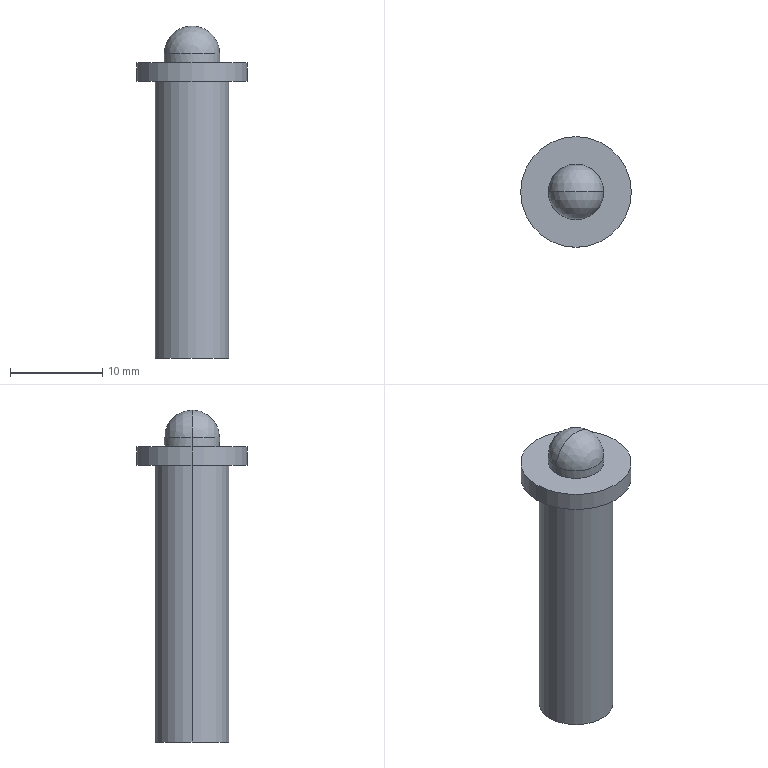Part | STEP file | 2055 Spring mounting seat B | 1 solid | 15 faces | box 12 x 12 x 36 mm | volume 1619 mm3 | cylinder 8 | plane 3 | cone 2 | sphere 2 | commonest cylinder face diameters 4.2 x2 6 x2 8 x2 12 x2
STEP:
#1=CARTESIAN_POINT('',(0.,0.,0.));
#2=DIRECTION('',(0.,0.,1.));
#3=DIRECTION('',(1.,0.,0.));
#4=AXIS2_PLACEMENT_3D('',#1,#2,#3);
#5=CARTESIAN_POINT('',(-2.1,0.,-18.));
#6=VERTEX_POINT('',#5);
#7=CARTESIAN_POINT('',(-2.1,0.,-32.));
#8=VERTEX_POINT('',#7);
#9=CARTESIAN_POINT('',(-2.1,0.,-32.));
#10=DIRECTION('',(0.,0.,-1.));
#11=VECTOR('',#10,1.);
#12=LINE('',#9,#11);
#13=CARTESIAN_POINT('',(0.,0.,-32.));
#14=DIRECTION('',(0.,0.,-1.));
#15=DIRECTION('',(-1.,0.,0.));
#16=AXIS2_PLACEMENT_3D('',#13,#14,#15);
#17=CYLINDRICAL_SURFACE('',#16,2.1);
#18=CARTESIAN_POINT('',(6.283,0.));
#19=DIRECTION('',(0.,1.));
#20=VECTOR('',#19,1.);
#21=LINE('',#18,#20);
#22=(GEOMETRIC_REPRESENTATION_CONTEXT(2)PARAMETRIC_REPRESENTATION_CONTEXT()REPRESENTATION_CONTEXT('',''));
#23=DEFINITIONAL_REPRESENTATION('',(#21),#22);
#24=PCURVE('',#17,#23);
#25=CARTESIAN_POINT('',(0.,0.,-32.));
#26=DIRECTION('',(0.,0.,-1.));
#27=DIRECTION('',(-1.,0.,0.));
#28=AXIS2_PLACEMENT_3D('',#25,#26,#27);
#29=CYLINDRICAL_SURFACE('',#28,2.1);
#30=CARTESIAN_POINT('',(0.,0.));
#31=DIRECTION('',(0.,1.));
#32=VECTOR('',#31,1.);
#33=LINE('',#30,#32);
#34=(GEOMETRIC_REPRESENTATION_CONTEXT(2)PARAMETRIC_REPRESENTATION_CONTEXT()REPRESENTATION_CONTEXT('',''));
#35=DEFINITIONAL_REPRESENTATION('',(#33),#34);
#36=PCURVE('',#29,#35);
#37=SURFACE_CURVE('',#12,(#24,#36),.PCURVE_S1.);
#38=EDGE_CURVE('',#6,#8,#37,.T.);
#39=ORIENTED_EDGE('',*,*,#38,.T.);
#40=CARTESIAN_POINT('',(2.1,0.,-32.));
#41=VERTEX_POINT('',#40);
#42=CARTESIAN_POINT('',(0.,0.,-32.));
#43=DIRECTION('',(0.,0.,-1.));
#44=DIRECTION('',(-1.,0.,0.));
#45=AXIS2_PLACEMENT_3D('',#42,#43,#44);
#46=CIRCLE('',#45,2.1);
#47=CARTESIAN_POINT('',(0.,0.));
#48=DIRECTION('',(1.,0.));
#49=VECTOR('',#48,1.);
#50=LINE('',#47,#49);
#51=(GEOMETRIC_REPRESENTATION_CONTEXT(2)PARAMETRIC_REPRESENTATION_CONTEXT()REPRESENTATION_CONTEXT('',''));
#52=DEFINITIONAL_REPRESENTATION('',(#50),#51);
#53=PCURVE('',#17,#52);
#54=CARTESIAN_POINT('',(0.,0.,-32.));
#55=DIRECTION('',(0.,0.,-1.));
#56=DIRECTION('',(-1.,0.,0.));
#57=AXIS2_PLACEMENT_3D('',#54,#55,#56);
#58=PLANE('',#57);
#59=CARTESIAN_POINT('',(0.,0.));
#60=DIRECTION('',(1.,0.));
#61=AXIS2_PLACEMENT_2D('',#59,#60);
#62=CIRCLE('',#61,2.1);
#63=(GEOMETRIC_REPRESENTATION_CONTEXT(2)PARAMETRIC_REPRESENTATION_CONTEXT()REPRESENTATION_CONTEXT('',''));
#64=DEFINITIONAL_REPRESENTATION('',(#62),#63);
#65=PCURVE('',#58,#64);
#66=SURFACE_CURVE('',#46,(#53,#65),.PCURVE_S1.);
#67=EDGE_CURVE('',#41,#8,#66,.T.);
#68=ORIENTED_EDGE('',*,*,#67,.F.);
#69=CARTESIAN_POINT('',(2.1,0.,-18.));
#70=VERTEX_POINT('',#69);
#71=CARTESIAN_POINT('',(2.1,0.,-32.));
#72=DIRECTION('',(0.,0.,-1.));
#73=VECTOR('',#72,1.);
#74=LINE('',#71,#73);
#75=CARTESIAN_POINT('',(3.142,0.));
#76=DIRECTION('',(0.,1.));
#77=VECTOR('',#76,1.);
#78=LINE('',#75,#77);
#79=(GEOMETRIC_REPRESENTATION_CONTEXT(2)PARAMETRIC_REPRESENTATION_CONTEXT()REPRESENTATION_CONTEXT('',''));
#80=DEFINITIONAL_REPRESENTATION('',(#78),#79);
#81=PCURVE('',#17,#80);
#82=CARTESIAN_POINT('',(3.142,0.));
#83=DIRECTION('',(0.,1.));
#84=VECTOR('',#83,1.);
#85=LINE('',#82,#84);
#86=(GEOMETRIC_REPRESENTATION_CONTEXT(2)PARAMETRIC_REPRESENTATION_CONTEXT()REPRESENTATION_CONTEXT('',''));
#87=DEFINITIONAL_REPRESENTATION('',(#85),#86);
#88=PCURVE('',#29,#87);
#89=SURFACE_CURVE('',#74,(#81,#88),.PCURVE_S1.);
#90=EDGE_CURVE('',#70,#41,#89,.T.);
#91=ORIENTED_EDGE('',*,*,#90,.F.);
#92=CARTESIAN_POINT('',(0.,0.,-18.));
#93=DIRECTION('',(0.,0.,-1.));
#94=DIRECTION('',(-1.,0.,0.));
#95=AXIS2_PLACEMENT_3D('',#92,#93,#94);
#96=CIRCLE('',#95,2.1);
#97=CARTESIAN_POINT('',(0.,-14.));
#98=DIRECTION('',(1.,0.));
#99=VECTOR('',#98,1.);
#100=LINE('',#97,#99);
#101=(GEOMETRIC_REPRESENTATION_CONTEXT(2)PARAMETRIC_REPRESENTATION_CONTEXT()REPRESENTATION_CONTEXT('',''));
#102=DEFINITIONAL_REPRESENTATION('',(#100),#101);
#103=PCURVE('',#17,#102);
#104=CARTESIAN_POINT('',(0.,0.,-18.));
#105=DIRECTION('',(0.,0.,-1.));
#106=DIRECTION('',(-1.,0.,0.));
#107=AXIS2_PLACEMENT_3D('',#104,#105,#106);
#108=CONICAL_SURFACE('',#107,2.1,1.03);
#109=CARTESIAN_POINT('',(0.,0.));
#110=DIRECTION('',(1.,0.));
#111=VECTOR('',#110,1.);
#112=LINE('',#109,#111);
#113=(GEOMETRIC_REPRESENTATION_CONTEXT(2)PARAMETRIC_REPRESENTATION_CONTEXT()REPRESENTATION_CONTEXT('',''));
#114=DEFINITIONAL_REPRESENTATION('',(#112),#113);
#115=PCURVE('',#108,#114);
#116=SURFACE_CURVE('',#96,(#103,#115),.PCURVE_S1.);
#117=EDGE_CURVE('',#70,#6,#116,.T.);
#118=ORIENTED_EDGE('',*,*,#117,.T.);
#119=EDGE_LOOP('',(#39,#68,#91,#118));
#120=FACE_BOUND('',#119,.F.);
#121=ADVANCED_FACE('',(#120),#17,.F.);
#122=ORIENTED_EDGE('',*,*,#117,.F.);
#123=CARTESIAN_POINT('',(0.,0.,-16.738));
#124=VERTEX_POINT('',#123);
#125=CARTESIAN_POINT('',(2.1,0.,-18.));
#126=DIRECTION('',(0.8572,0.,-0.515));
#127=VECTOR('',#126,1.);
#128=LINE('',#125,#127);
#129=CARTESIAN_POINT('',(3.142,-1.262));
#130=CARTESIAN_POINT('',(3.142,-1.243));
#131=CARTESIAN_POINT('',(3.142,-1.204));
#132=CARTESIAN_POINT('',(3.142,-1.147));
#133=CARTESIAN_POINT('',(3.142,-1.09));
#134=CARTESIAN_POINT('',(3.142,-1.032));
#135=CARTESIAN_POINT('',(3.142,-0.975));
#136=CARTESIAN_POINT('',(3.142,-0.9177));
#137=CARTESIAN_POINT('',(3.142,-0.8603));
#138=CARTESIAN_POINT('',(3.142,-0.803));
#139=CARTESIAN_POINT('',(3.142,-0.7456));
#140=CARTESIAN_POINT('',(3.142,-0.6883));
#141=CARTESIAN_POINT('',(3.142,-0.6309));
#142=CARTESIAN_POINT('',(3.142,-0.5735));
#143=CARTESIAN_POINT('',(3.142,-0.5162));
#144=CARTESIAN_POINT('',(3.142,-0.4588));
#145=CARTESIAN_POINT('',(3.142,-0.4015));
#146=CARTESIAN_POINT('',(3.142,-0.3441));
#147=CARTESIAN_POINT('',(3.142,-0.2868));
#148=CARTESIAN_POINT('',(3.142,-0.2294));
#149=CARTESIAN_POINT('',(3.142,-0.1721));
#150=CARTESIAN_POINT('',(3.142,-0.1147));
#151=CARTESIAN_POINT('',(3.142,-0.05735));
#152=CARTESIAN_POINT('',(3.142,-0.01912));
#153=CARTESIAN_POINT('',(3.142,0.));
#154=B_SPLINE_CURVE_WITH_KNOTS('',3,(#129,#130,#131,#132,#133,#134,#135,#136,#137,#138,#139,#140,#141,#142,#143,#144,#145,#146,#147,#148,#149,#150,#151,#152,#153),.UNSPECIFIED.,.F.,.F.,(4,1,1,1,1,1,1,1,1,1,1,1,1,1,1,1,1,1,1,1,1,1,4),(-2.45,-2.339,-2.227,-2.116,-2.004,-1.893,-1.782,-1.67,-1.559,-1.448,-1.336,-1.225,-1.114,-1.002,-0.8909,-0.7795,-0.6682,-0.5568,-0.4454,-0.3341,-0.2227,-0.1114,0.),.QUASI_UNIFORM_KNOTS.);
#155=(GEOMETRIC_REPRESENTATION_CONTEXT(2)PARAMETRIC_REPRESENTATION_CONTEXT()REPRESENTATION_CONTEXT('',''));
#156=DEFINITIONAL_REPRESENTATION('',(#154),#155);
#157=PCURVE('',#108,#156);
#158=CARTESIAN_POINT('',(0.,0.,-18.));
#159=DIRECTION('',(0.,0.,-1.));
#160=DIRECTION('',(-1.,0.,0.));
#161=AXIS2_PLACEMENT_3D('',#158,#159,#160);
#162=CONICAL_SURFACE('',#161,2.1,1.03);
#163=CARTESIAN_POINT('',(3.142,-1.262));
#164=CARTESIAN_POINT('',(3.142,-1.243));
#165=CARTESIAN_POINT('',(3.142,-1.204));
#166=CARTESIAN_POINT('',(3.142,-1.147));
#167=CARTESIAN_POINT('',(3.142,-1.09));
#168=CARTESIAN_POINT('',(3.142,-1.032));
#169=CARTESIAN_POINT('',(3.142,-0.975));
#170=CARTESIAN_POINT('',(3.142,-0.9177));
#171=CARTESIAN_POINT('',(3.142,-0.8603));
#172=CARTESIAN_POINT('',(3.142,-0.803));
#173=CARTESIAN_POINT('',(3.142,-0.7456));
#174=CARTESIAN_POINT('',(3.142,-0.6883));
#175=CARTESIAN_POINT('',(3.142,-0.6309));
#176=CARTESIAN_POINT('',(3.142,-0.5735));
#177=CARTESIAN_POINT('',(3.142,-0.5162));
#178=CARTESIAN_POINT('',(3.142,-0.4588));
#179=CARTESIAN_POINT('',(3.142,-0.4015));
#180=CARTESIAN_POINT('',(3.142,-0.3441));
#181=CARTESIAN_POINT('',(3.142,-0.2868));
#182=CARTESIAN_POINT('',(3.142,-0.2294));
#183=CARTESIAN_POINT('',(3.142,-0.1721));
#184=CARTESIAN_POINT('',(3.142,-0.1147));
#185=CARTESIAN_POINT('',(3.142,-0.05735));
#186=CARTESIAN_POINT('',(3.142,-0.01912));
#187=CARTESIAN_POINT('',(3.142,0.));
#188=B_SPLINE_CURVE_WITH_KNOTS('',3,(#163,#164,#165,#166,#167,#168,#169,#170,#171,#172,#173,#174,#175,#176,#177,#178,#179,#180,#181,#182,#183,#184,#185,#186,#187),.UNSPECIFIED.,.F.,.F.,(4,1,1,1,1,1,1,1,1,1,1,1,1,1,1,1,1,1,1,1,1,1,4),(-2.45,-2.339,-2.227,-2.116,-2.004,-1.893,-1.782,-1.67,-1.559,-1.448,-1.336,-1.225,-1.114,-1.002,-0.8909,-0.7795,-0.6682,-0.5568,-0.4454,-0.3341,-0.2227,-0.1114,0.),.QUASI_UNIFORM_KNOTS.);
#189=(GEOMETRIC_REPRESENTATION_CONTEXT(2)PARAMETRIC_REPRESENTATION_CONTEXT()REPRESENTATION_CONTEXT('',''));
#190=DEFINITIONAL_REPRESENTATION('',(#188),#189);
#191=PCURVE('',#162,#190);
#192=SURFACE_CURVE('',#128,(#157,#191),.PCURVE_S1.);
#193=EDGE_CURVE('',#124,#70,#192,.T.);
#194=ORIENTED_EDGE('',*,*,#193,.F.);
#195=CARTESIAN_POINT('',(-2.1,0.,-18.));
#196=DIRECTION('',(-0.8572,0.,-0.515));
#197=VECTOR('',#196,1.);
#198=LINE('',#195,#197);
#199=CARTESIAN_POINT('',(6.283,0.));
#200=DIRECTION('',(0.,1.));
#201=VECTOR('',#200,1.);
#202=LINE('',#199,#201);
#203=(GEOMETRIC_REPRESENTATION_CONTEXT(2)PARAMETRIC_REPRESENTATION_CONTEXT()REPRESENTATION_CONTEXT('',''));
#204=DEFINITIONAL_REPRESENTATION('',(#202),#203);
#205=PCURVE('',#108,#204);
#206=CARTESIAN_POINT('',(0.,0.));
#207=DIRECTION('',(0.,1.));
#208=VECTOR('',#207,1.);
#209=LINE('',#206,#208);
#210=(GEOMETRIC_REPRESENTATION_CONTEXT(2)PARAMETRIC_REPRESENTATION_CONTEXT()REPRESENTATION_CONTEXT('',''));
#211=DEFINITIONAL_REPRESENTATION('',(#209),#210);
#212=PCURVE('',#162,#211);
#213=SURFACE_CURVE('',#198,(#205,#212),.PCURVE_S1.);
#214=EDGE_CURVE('',#124,#6,#213,.T.);
#215=ORIENTED_EDGE('',*,*,#214,.T.);
#216=EDGE_LOOP('',(#122,#194,#215));
#217=FACE_BOUND('',#216,.F.);
#218=ADVANCED_FACE('',(#217),#108,.F.);
#219=CARTESIAN_POINT('',(0.,3.,1.));
#220=VERTEX_POINT('',#219);
#221=CARTESIAN_POINT('',(3.,0.,1.));
#222=VERTEX_POINT('',#221);
#223=CARTESIAN_POINT('',(0.,0.,1.));
#224=DIRECTION('',(0.,0.,-1.));
#225=DIRECTION('',(-1.,0.,0.));
#226=AXIS2_PLACEMENT_3D('',#223,#224,#225);
#227=CIRCLE('',#226,3.);
#228=CARTESIAN_POINT('',(0.,0.,1.));
#229=DIRECTION('',(0.,1.,0.));
#230=DIRECTION('',(1.,0.,0.));
#231=AXIS2_PLACEMENT_3D('',#228,#229,#230);
#232=SPHERICAL_SURFACE('',#231,3.);
#233=CARTESIAN_POINT('',(6.283,1.571));
#234=CARTESIAN_POINT('',(6.283,1.547));
#235=CARTESIAN_POINT('',(6.283,1.499));
#236=CARTESIAN_POINT('',(6.283,1.428));
#237=CARTESIAN_POINT('',(6.283,1.357));
#238=CARTESIAN_POINT('',(6.283,1.285));
#239=CARTESIAN_POINT('',(6.283,1.214));
#240=CARTESIAN_POINT('',(6.283,1.142));
#241=CARTESIAN_POINT('',(6.283,1.071));
#242=CARTESIAN_POINT('',(6.283,0.9996));
#243=CARTESIAN_POINT('',(6.283,0.9282));
#244=CARTESIAN_POINT('',(6.283,0.8568));
#245=CARTESIAN_POINT('',(6.283,0.7854));
#246=CARTESIAN_POINT('',(6.283,0.714));
#247=CARTESIAN_POINT('',(6.283,0.6426));
#248=CARTESIAN_POINT('',(6.283,0.5712));
#249=CARTESIAN_POINT('',(6.283,0.4998));
#250=CARTESIAN_POINT('',(6.283,0.4284));
#251=CARTESIAN_POINT('',(6.283,0.357));
#252=CARTESIAN_POINT('',(6.283,0.2856));
#253=CARTESIAN_POINT('',(6.283,0.2142));
#254=CARTESIAN_POINT('',(6.283,0.1428));
#255=CARTESIAN_POINT('',(6.283,0.0714));
#256=CARTESIAN_POINT('',(6.283,0.0238));
#257=CARTESIAN_POINT('',(6.283,0.));
#258=B_SPLINE_CURVE_WITH_KNOTS('',3,(#233,#234,#235,#236,#237,#238,#239,#240,#241,#242,#243,#244,#245,#246,#247,#248,#249,#250,#251,#252,#253,#254,#255,#256,#257),.UNSPECIFIED.,.F.,.F.,(4,1,1,1,1,1,1,1,1,1,1,1,1,1,1,1,1,1,1,1,1,1,4),(1.571,1.642,1.714,1.785,1.856,1.928,1.999,2.071,2.142,2.213,2.285,2.356,2.428,2.499,2.57,2.642,2.713,2.785,2.856,2.927,2.999,3.07,3.142),.QUASI_UNIFORM_KNOTS.);
#259=(GEOMETRIC_REPRESENTATION_CONTEXT(2)PARAMETRIC_REPRESENTATION_CONTEXT()REPRESENTATION_CONTEXT('',''));
#260=DEFINITIONAL_REPRESENTATION('',(#258),#259);
#261=PCURVE('',#232,#260);
#262=CARTESIAN_POINT('',(0.,0.,4.));
#263=DIRECTION('',(0.,0.,-1.));
#264=DIRECTION('',(-1.,0.,0.));
#265=AXIS2_PLACEMENT_3D('',#262,#263,#264);
#266=CYLINDRICAL_SURFACE('',#265,3.);
#267=CARTESIAN_POINT('',(0.,3.));
#268=DIRECTION('',(1.,0.));
#269=VECTOR('',#268,1.);
#270=LINE('',#267,#269);
#271=(GEOMETRIC_REPRESENTATION_CONTEXT(2)PARAMETRIC_REPRESENTATION_CONTEXT()REPRESENTATION_CONTEXT('',''));
#272=DEFINITIONAL_REPRESENTATION('',(#270),#271);
#273=PCURVE('',#266,#272);
#274=SURFACE_CURVE('',#227,(#261,#273),.PCURVE_S1.);
#275=EDGE_CURVE('',#220,#222,#274,.T.);
#276=ORIENTED_EDGE('',*,*,#275,.F.);
#277=CARTESIAN_POINT('',(-3.,0.,1.));
#278=VERTEX_POINT('',#277);
#279=CARTESIAN_POINT('',(0.,0.,1.));
#280=DIRECTION('',(0.,0.,-1.));
#281=DIRECTION('',(-1.,0.,0.));
#282=AXIS2_PLACEMENT_3D('',#279,#280,#281);
#283=CIRCLE('',#282,3.);
#284=CARTESIAN_POINT('',(3.142,0.));
#285=DIRECTION('',(0.,1.));
#286=VECTOR('',#285,1.);
#287=LINE('',#284,#286);
#288=(GEOMETRIC_REPRESENTATION_CONTEXT(2)PARAMETRIC_REPRESENTATION_CONTEXT()REPRESENTATION_CONTEXT('',''));
#289=DEFINITIONAL_REPRESENTATION('',(#287),#288);
#290=PCURVE('',#232,#289);
#291=CARTESIAN_POINT('',(0.,3.));
#292=DIRECTION('',(1.,0.));
#293=VECTOR('',#292,1.);
#294=LINE('',#291,#293);
#295=(GEOMETRIC_REPRESENTATION_CONTEXT(2)PARAMETRIC_REPRESENTATION_CONTEXT()REPRESENTATION_CONTEXT('',''));
#296=DEFINITIONAL_REPRESENTATION('',(#294),#295);
#297=PCURVE('',#266,#296);
#298=SURFACE_CURVE('',#283,(#290,#297),.PCURVE_S1.);
#299=EDGE_CURVE('',#278,#220,#298,.T.);
#300=ORIENTED_EDGE('',*,*,#299,.F.);
#301=CARTESIAN_POINT('',(0.,0.,4.));
#302=VERTEX_POINT('',#301);
#303=CARTESIAN_POINT('',(0.,0.,1.));
#304=DIRECTION('',(0.,1.,0.));
#305=DIRECTION('',(-1.,0.,0.));
#306=AXIS2_PLACEMENT_3D('',#303,#304,#305);
#307=CIRCLE('',#306,3.);
#308=CARTESIAN_POINT('',(3.142,0.));
#309=DIRECTION('',(1.,0.));
#310=VECTOR('',#309,1.);
#311=LINE('',#308,#310);
#312=(GEOMETRIC_REPRESENTATION_CONTEXT(2)PARAMETRIC_REPRESENTATION_CONTEXT()REPRESENTATION_CONTEXT('',''));
#313=DEFINITIONAL_REPRESENTATION('',(#311),#312);
#314=PCURVE('',#232,#313);
#315=CARTESIAN_POINT('',(0.,0.,1.));
#316=DIRECTION('',(0.,1.,0.));
#317=DIRECTION('',(1.,0.,0.));
#318=AXIS2_PLACEMENT_3D('',#315,#316,#317);
#319=SPHERICAL_SURFACE('',#318,3.);
#320=CARTESIAN_POINT('',(3.142,0.));
#321=DIRECTION('',(1.,0.));
#322=VECTOR('',#321,1.);
#323=LINE('',#320,#322);
#324=(GEOMETRIC_REPRESENTATION_CONTEXT(2)PARAMETRIC_REPRESENTATION_CONTEXT()REPRESENTATION_CONTEXT('',''));
#325=DEFINITIONAL_REPRESENTATION('',(#323),#324);
#326=PCURVE('',#319,#325);
#327=SURFACE_CURVE('',#307,(#314,#326),.PCURVE_S1.);
#328=EDGE_CURVE('',#278,#302,#327,.T.);
#329=ORIENTED_EDGE('',*,*,#328,.T.);
#330=CARTESIAN_POINT('',(0.,0.,1.));
#331=DIRECTION('',(0.,-1.,0.));
#332=DIRECTION('',(0.,0.,-1.));
#333=AXIS2_PLACEMENT_3D('',#330,#331,#332);
#334=CIRCLE('',#333,3.);
#335=CARTESIAN_POINT('',(6.283,0.));
#336=CARTESIAN_POINT('',(6.259,0.));
#337=CARTESIAN_POINT('',(6.212,0.));
#338=CARTESIAN_POINT('',(6.14,0.));
#339=CARTESIAN_POINT('',(6.069,0.));
#340=CARTESIAN_POINT('',(5.998,0.));
#341=CARTESIAN_POINT('',(5.926,0.));
#342=CARTESIAN_POINT('',(5.855,0.));
#343=CARTESIAN_POINT('',(5.783,0.));
#344=CARTESIAN_POINT('',(5.712,0.));
#345=CARTESIAN_POINT('',(5.641,0.));
#346=CARTESIAN_POINT('',(5.569,0.));
#347=CARTESIAN_POINT('',(5.498,0.));
#348=CARTESIAN_POINT('',(5.426,0.));
#349=CARTESIAN_POINT('',(5.355,0.));
#350=CARTESIAN_POINT('',(5.284,0.));
#351=CARTESIAN_POINT('',(5.212,0.));
#352=CARTESIAN_POINT('',(5.141,0.));
#353=CARTESIAN_POINT('',(5.069,0.));
#354=CARTESIAN_POINT('',(4.998,0.));
#355=CARTESIAN_POINT('',(4.927,0.));
#356=CARTESIAN_POINT('',(4.855,0.));
#357=CARTESIAN_POINT('',(4.784,0.));
#358=CARTESIAN_POINT('',(4.736,0.));
#359=CARTESIAN_POINT('',(4.712,0.));
#360=B_SPLINE_CURVE_WITH_KNOTS('',3,(#335,#336,#337,#338,#339,#340,#341,#342,#343,#344,#345,#346,#347,#348,#349,#350,#351,#352,#353,#354,#355,#356,#357,#358,#359),.UNSPECIFIED.,.F.,.F.,(4,1,1,1,1,1,1,1,1,1,1,1,1,1,1,1,1,1,1,1,1,1,4),(1.571,1.642,1.714,1.785,1.856,1.928,1.999,2.071,2.142,2.213,2.285,2.356,2.428,2.499,2.57,2.642,2.713,2.785,2.856,2.927,2.999,3.07,3.142),.QUASI_UNIFORM_KNOTS.);
#361=(GEOMETRIC_REPRESENTATION_CONTEXT(2)PARAMETRIC_REPRESENTATION_CONTEXT()REPRESENTATION_CONTEXT('',''));
#362=DEFINITIONAL_REPRESENTATION('',(#360),#361);
#363=PCURVE('',#232,#362);
#364=CARTESIAN_POINT('',(6.283,0.));
#365=CARTESIAN_POINT('',(6.259,0.));
#366=CARTESIAN_POINT('',(6.212,0.));
#367=CARTESIAN_POINT('',(6.14,0.));
#368=CARTESIAN_POINT('',(6.069,0.));
#369=CARTESIAN_POINT('',(5.998,0.));
#370=CARTESIAN_POINT('',(5.926,0.));
#371=CARTESIAN_POINT('',(5.855,0.));
#372=CARTESIAN_POINT('',(5.783,0.));
#373=CARTESIAN_POINT('',(5.712,0.));
#374=CARTESIAN_POINT('',(5.641,0.));
#375=CARTESIAN_POINT('',(5.569,0.));
#376=CARTESIAN_POINT('',(5.498,0.));
#377=CARTESIAN_POINT('',(5.426,0.));
#378=CARTESIAN_POINT('',(5.355,0.));
#379=CARTESIAN_POINT('',(5.284,0.));
#380=CARTESIAN_POINT('',(5.212,0.));
#381=CARTESIAN_POINT('',(5.141,0.));
#382=CARTESIAN_POINT('',(5.069,0.));
#383=CARTESIAN_POINT('',(4.998,0.));
#384=CARTESIAN_POINT('',(4.927,0.));
#385=CARTESIAN_POINT('',(4.855,0.));
#386=CARTESIAN_POINT('',(4.784,0.));
#387=CARTESIAN_POINT('',(4.736,0.));
#388=CARTESIAN_POINT('',(4.712,0.));
#389=B_SPLINE_CURVE_WITH_KNOTS('',3,(#364,#365,#366,#367,#368,#369,#370,#371,#372,#373,#374,#375,#376,#377,#378,#379,#380,#381,#382,#383,#384,#385,#386,#387,#388),.UNSPECIFIED.,.F.,.F.,(4,1,1,1,1,1,1,1,1,1,1,1,1,1,1,1,1,1,1,1,1,1,4),(1.571,1.642,1.714,1.785,1.856,1.928,1.999,2.071,2.142,2.213,2.285,2.356,2.428,2.499,2.57,2.642,2.713,2.785,2.856,2.927,2.999,3.07,3.142),.QUASI_UNIFORM_KNOTS.);
#390=(GEOMETRIC_REPRESENTATION_CONTEXT(2)PARAMETRIC_REPRESENTATION_CONTEXT()REPRESENTATION_CONTEXT('',''));
#391=DEFINITIONAL_REPRESENTATION('',(#389),#390);
#392=PCURVE('',#319,#391);
#393=SURFACE_CURVE('',#334,(#363,#392),.PCURVE_S1.);
#394=EDGE_CURVE('',#222,#302,#393,.T.);
#395=ORIENTED_EDGE('',*,*,#394,.F.);
#396=EDGE_LOOP('',(#276,#300,#329,#395));
#397=FACE_BOUND('',#396,.T.);
#398=ADVANCED_FACE('',(#397),#232,.T.);
#399=CARTESIAN_POINT('',(-4.,0.,-32.));
#400=VERTEX_POINT('',#399);
#401=CARTESIAN_POINT('',(4.,0.,-32.));
#402=VERTEX_POINT('',#401);
#403=CARTESIAN_POINT('',(0.,0.,-32.));
#404=DIRECTION('',(0.,0.,-1.));
#405=DIRECTION('',(-1.,0.,0.));
#406=AXIS2_PLACEMENT_3D('',#403,#404,#405);
#407=CIRCLE('',#406,4.);
#408=CARTESIAN_POINT('',(0.,0.,-32.));
#409=DIRECTION('',(0.,0.,1.));
#410=DIRECTION('',(1.,0.,0.));
#411=AXIS2_PLACEMENT_3D('',#408,#409,#410);
#412=CYLINDRICAL_SURFACE('',#411,4.);
#413=CARTESIAN_POINT('',(3.142,0.));
#414=DIRECTION('',(-1.,0.));
#415=VECTOR('',#414,1.);
#416=LINE('',#413,#415);
#417=(GEOMETRIC_REPRESENTATION_CONTEXT(2)PARAMETRIC_REPRESENTATION_CONTEXT()REPRESENTATION_CONTEXT('',''));
#418=DEFINITIONAL_REPRESENTATION('',(#416),#417);
#419=PCURVE('',#412,#418);
#420=CARTESIAN_POINT('',(0.,0.));
#421=DIRECTION('',(1.,0.));
#422=AXIS2_PLACEMENT_2D('',#420,#421);
#423=CIRCLE('',#422,4.);
#424=(GEOMETRIC_REPRESENTATION_CONTEXT(2)PARAMETRIC_REPRESENTATION_CONTEXT()REPRESENTATION_CONTEXT('',''));
#425=DEFINITIONAL_REPRESENTATION('',(#423),#424);
#426=PCURVE('',#58,#425);
#427=SURFACE_CURVE('',#407,(#419,#426),.PCURVE_S1.);
#428=EDGE_CURVE('',#400,#402,#427,.T.);
#429=ORIENTED_EDGE('',*,*,#428,.F.);
#430=CARTESIAN_POINT('',(-4.,0.,-2.));
#431=VERTEX_POINT('',#430);
#432=CARTESIAN_POINT('',(-4.,0.,-32.));
#433=DIRECTION('',(0.,0.,1.));
#434=VECTOR('',#433,1.);
#435=LINE('',#432,#434);
#436=CARTESIAN_POINT('',(3.142,0.));
#437=DIRECTION('',(0.,1.));
#438=VECTOR('',#437,1.);
#439=LINE('',#436,#438);
#440=(GEOMETRIC_REPRESENTATION_CONTEXT(2)PARAMETRIC_REPRESENTATION_CONTEXT()REPRESENTATION_CONTEXT('',''));
#441=DEFINITIONAL_REPRESENTATION('',(#439),#440);
#442=PCURVE('',#412,#441);
#443=CARTESIAN_POINT('',(0.,0.,-32.));
#444=DIRECTION('',(0.,0.,1.));
#445=DIRECTION('',(1.,0.,0.));
#446=AXIS2_PLACEMENT_3D('',#443,#444,#445);
#447=CYLINDRICAL_SURFACE('',#446,4.);
#448=CARTESIAN_POINT('',(3.142,0.));
#449=DIRECTION('',(0.,1.));
#450=VECTOR('',#449,1.);
#451=LINE('',#448,#450);
#452=(GEOMETRIC_REPRESENTATION_CONTEXT(2)PARAMETRIC_REPRESENTATION_CONTEXT()REPRESENTATION_CONTEXT('',''));
#453=DEFINITIONAL_REPRESENTATION('',(#451),#452);
#454=PCURVE('',#447,#453);
#455=SURFACE_CURVE('',#435,(#442,#454),.PCURVE_S1.);
#456=EDGE_CURVE('',#400,#431,#455,.T.);
#457=ORIENTED_EDGE('',*,*,#456,.T.);
#458=CARTESIAN_POINT('',(4.,0.,-2.));
#459=VERTEX_POINT('',#458);
#460=CARTESIAN_POINT('',(0.,0.,-2.));
#461=DIRECTION('',(0.,0.,-1.));
#462=DIRECTION('',(-1.,0.,0.));
#463=AXIS2_PLACEMENT_3D('',#460,#461,#462);
#464=CIRCLE('',#463,4.);
#465=CARTESIAN_POINT('',(3.142,30.));
#466=DIRECTION('',(-1.,0.));
#467=VECTOR('',#466,1.);
#468=LINE('',#465,#467);
#469=(GEOMETRIC_REPRESENTATION_CONTEXT(2)PARAMETRIC_REPRESENTATION_CONTEXT()REPRESENTATION_CONTEXT('',''));
#470=DEFINITIONAL_REPRESENTATION('',(#468),#469);
#471=PCURVE('',#412,#470);
#472=CARTESIAN_POINT('',(0.,0.,-2.));
#473=DIRECTION('',(0.,0.,-1.));
#474=DIRECTION('',(-1.,0.,0.));
#475=AXIS2_PLACEMENT_3D('',#472,#473,#474);
#476=PLANE('',#475);
#477=CARTESIAN_POINT('',(0.,0.));
#478=DIRECTION('',(1.,0.));
#479=AXIS2_PLACEMENT_2D('',#477,#478);
#480=CIRCLE('',#479,4.);
#481=(GEOMETRIC_REPRESENTATION_CONTEXT(2)PARAMETRIC_REPRESENTATION_CONTEXT()REPRESENTATION_CONTEXT('',''));
#482=DEFINITIONAL_REPRESENTATION('',(#480),#481);
#483=PCURVE('',#476,#482);
#484=SURFACE_CURVE('',#464,(#471,#483),.PCURVE_S1.);
#485=EDGE_CURVE('',#431,#459,#484,.T.);
#486=ORIENTED_EDGE('',*,*,#485,.T.);
#487=CARTESIAN_POINT('',(4.,0.,-32.));
#488=DIRECTION('',(0.,0.,1.));
#489=VECTOR('',#488,1.);
#490=LINE('',#487,#489);
#491=CARTESIAN_POINT('',(0.,0.));
#492=DIRECTION('',(0.,1.));
#493=VECTOR('',#492,1.);
#494=LINE('',#491,#493);
#495=(GEOMETRIC_REPRESENTATION_CONTEXT(2)PARAMETRIC_REPRESENTATION_CONTEXT()REPRESENTATION_CONTEXT('',''));
#496=DEFINITIONAL_REPRESENTATION('',(#494),#495);
#497=PCURVE('',#412,#496);
#498=CARTESIAN_POINT('',(6.283,0.));
#499=DIRECTION('',(0.,1.));
#500=VECTOR('',#499,1.);
#501=LINE('',#498,#500);
#502=(GEOMETRIC_REPRESENTATION_CONTEXT(2)PARAMETRIC_REPRESENTATION_CONTEXT()REPRESENTATION_CONTEXT('',''));
#503=DEFINITIONAL_REPRESENTATION('',(#501),#502);
#504=PCURVE('',#447,#503);
#505=SURFACE_CURVE('',#490,(#497,#504),.PCURVE_S1.);
#506=EDGE_CURVE('',#402,#459,#505,.T.);
#507=ORIENTED_EDGE('',*,*,#506,.F.);
#508=EDGE_LOOP('',(#429,#457,#486,#507));
#509=FACE_BOUND('',#508,.T.);
#510=ADVANCED_FACE('',(#509),#412,.T.);
#511=CARTESIAN_POINT('',(-6.,0.,-2.));
#512=VERTEX_POINT('',#511);
#513=CARTESIAN_POINT('',(6.,0.,-2.));
#514=VERTEX_POINT('',#513);
#515=CARTESIAN_POINT('',(0.,0.,-2.));
#516=DIRECTION('',(0.,0.,-1.));
#517=DIRECTION('',(-1.,0.,0.));
#518=AXIS2_PLACEMENT_3D('',#515,#516,#517);
#519=CIRCLE('',#518,6.);
#520=CARTESIAN_POINT('',(0.,0.,-2.));
#521=DIRECTION('',(0.,0.,1.));
#522=DIRECTION('',(1.,0.,0.));
#523=AXIS2_PLACEMENT_3D('',#520,#521,#522);
#524=CYLINDRICAL_SURFACE('',#523,6.);
#525=CARTESIAN_POINT('',(3.142,0.));
#526=DIRECTION('',(-1.,0.));
#527=VECTOR('',#526,1.);
#528=LINE('',#525,#527);
#529=(GEOMETRIC_REPRESENTATION_CONTEXT(2)PARAMETRIC_REPRESENTATION_CONTEXT()REPRESENTATION_CONTEXT('',''));
#530=DEFINITIONAL_REPRESENTATION('',(#528),#529);
#531=PCURVE('',#524,#530);
#532=CARTESIAN_POINT('',(0.,0.));
#533=DIRECTION('',(1.,0.));
#534=AXIS2_PLACEMENT_2D('',#532,#533);
#535=CIRCLE('',#534,6.);
#536=(GEOMETRIC_REPRESENTATION_CONTEXT(2)PARAMETRIC_REPRESENTATION_CONTEXT()REPRESENTATION_CONTEXT('',''));
#537=DEFINITIONAL_REPRESENTATION('',(#535),#536);
#538=PCURVE('',#476,#537);
#539=SURFACE_CURVE('',#519,(#531,#538),.PCURVE_S1.);
#540=EDGE_CURVE('',#512,#514,#539,.T.);
#541=ORIENTED_EDGE('',*,*,#540,.F.);
#542=CARTESIAN_POINT('',(-6.,0.,0.));
#543=VERTEX_POINT('',#542);
#544=CARTESIAN_POINT('',(-6.,0.,-2.));
#545=DIRECTION('',(0.,0.,1.));
#546=VECTOR('',#545,1.);
#547=LINE('',#544,#546);
#548=CARTESIAN_POINT('',(3.142,0.));
#549=DIRECTION('',(0.,1.));
#550=VECTOR('',#549,1.);
#551=LINE('',#548,#550);
#552=(GEOMETRIC_REPRESENTATION_CONTEXT(2)PARAMETRIC_REPRESENTATION_CONTEXT()REPRESENTATION_CONTEXT('',''));
#553=DEFINITIONAL_REPRESENTATION('',(#551),#552);
#554=PCURVE('',#524,#553);
#555=CARTESIAN_POINT('',(0.,0.,-2.));
#556=DIRECTION('',(0.,0.,1.));
#557=DIRECTION('',(1.,0.,0.));
#558=AXIS2_PLACEMENT_3D('',#555,#556,#557);
#559=CYLINDRICAL_SURFACE('',#558,6.);
#560=CARTESIAN_POINT('',(3.142,0.));
#561=DIRECTION('',(0.,1.));
#562=VECTOR('',#561,1.);
#563=LINE('',#560,#562);
#564=(GEOMETRIC_REPRESENTATION_CONTEXT(2)PARAMETRIC_REPRESENTATION_CONTEXT()REPRESENTATION_CONTEXT('',''));
#565=DEFINITIONAL_REPRESENTATION('',(#563),#564);
#566=PCURVE('',#559,#565);
#567=SURFACE_CURVE('',#547,(#554,#566),.PCURVE_S1.);
#568=EDGE_CURVE('',#512,#543,#567,.T.);
#569=ORIENTED_EDGE('',*,*,#568,.T.);
#570=CARTESIAN_POINT('',(6.,0.,0.));
#571=VERTEX_POINT('',#570);
#572=CARTESIAN_POINT('',(0.,0.,0.));
#573=DIRECTION('',(0.,0.,-1.));
#574=DIRECTION('',(-1.,0.,0.));
#575=AXIS2_PLACEMENT_3D('',#572,#573,#574);
#576=CIRCLE('',#575,6.);
#577=CARTESIAN_POINT('',(3.142,2.));
#578=DIRECTION('',(-1.,0.));
#579=VECTOR('',#578,1.);
#580=LINE('',#577,#579);
#581=(GEOMETRIC_REPRESENTATION_CONTEXT(2)PARAMETRIC_REPRESENTATION_CONTEXT()REPRESENTATION_CONTEXT('',''));
#582=DEFINITIONAL_REPRESENTATION('',(#580),#581);
#583=PCURVE('',#524,#582);
#584=CARTESIAN_POINT('',(0.,0.,0.));
#585=DIRECTION('',(0.,0.,-1.));
#586=DIRECTION('',(-1.,0.,0.));
#587=AXIS2_PLACEMENT_3D('',#584,#585,#586);
#588=PLANE('',#587);
#589=CARTESIAN_POINT('',(0.,0.));
#590=DIRECTION('',(1.,0.));
#591=AXIS2_PLACEMENT_2D('',#589,#590);
#592=CIRCLE('',#591,6.);
#593=(GEOMETRIC_REPRESENTATION_CONTEXT(2)PARAMETRIC_REPRESENTATION_CONTEXT()REPRESENTATION_CONTEXT('',''));
#594=DEFINITIONAL_REPRESENTATION('',(#592),#593);
#595=PCURVE('',#588,#594);
#596=SURFACE_CURVE('',#576,(#583,#595),.PCURVE_S1.);
#597=EDGE_CURVE('',#543,#571,#596,.T.);
#598=ORIENTED_EDGE('',*,*,#597,.T.);
#599=CARTESIAN_POINT('',(6.,0.,-2.));
#600=DIRECTION('',(0.,0.,1.));
#601=VECTOR('',#600,1.);
#602=LINE('',#599,#601);
#603=CARTESIAN_POINT('',(0.,0.));
#604=DIRECTION('',(0.,1.));
#605=VECTOR('',#604,1.);
#606=LINE('',#603,#605);
#607=(GEOMETRIC_REPRESENTATION_CONTEXT(2)PARAMETRIC_REPRESENTATION_CONTEXT()REPRESENTATION_CONTEXT('',''));
#608=DEFINITIONAL_REPRESENTATION('',(#606),#607);
#609=PCURVE('',#524,#608);
#610=CARTESIAN_POINT('',(6.283,0.));
#611=DIRECTION('',(0.,1.));
#612=VECTOR('',#611,1.);
#613=LINE('',#610,#612);
#614=(GEOMETRIC_REPRESENTATION_CONTEXT(2)PARAMETRIC_REPRESENTATION_CONTEXT()REPRESENTATION_CONTEXT('',''));
#615=DEFINITIONAL_REPRESENTATION('',(#613),#614);
#616=PCURVE('',#559,#615);
#617=SURFACE_CURVE('',#602,(#609,#616),.PCURVE_S1.);
#618=EDGE_CURVE('',#514,#571,#617,.T.);
#619=ORIENTED_EDGE('',*,*,#618,.F.);
#620=EDGE_LOOP('',(#541,#569,#598,#619));
#621=FACE_BOUND('',#620,.T.);
#622=ADVANCED_FACE('',(#621),#524,.T.);
#623=ORIENTED_EDGE('',*,*,#275,.T.);
#624=CARTESIAN_POINT('',(3.,0.,0.));
#625=VERTEX_POINT('',#624);
#626=CARTESIAN_POINT('',(3.,0.,4.));
#627=DIRECTION('',(0.,0.,-1.));
#628=VECTOR('',#627,1.);
#629=LINE('',#626,#628);
#630=CARTESIAN_POINT('',(3.142,0.));
#631=DIRECTION('',(0.,1.));
#632=VECTOR('',#631,1.);
#633=LINE('',#630,#632);
#634=(GEOMETRIC_REPRESENTATION_CONTEXT(2)PARAMETRIC_REPRESENTATION_CONTEXT()REPRESENTATION_CONTEXT('',''));
#635=DEFINITIONAL_REPRESENTATION('',(#633),#634);
#636=PCURVE('',#266,#635);
#637=CARTESIAN_POINT('',(0.,0.,4.));
#638=DIRECTION('',(0.,0.,-1.));
#639=DIRECTION('',(-1.,0.,0.));
#640=AXIS2_PLACEMENT_3D('',#637,#638,#639);
#641=CYLINDRICAL_SURFACE('',#640,3.);
#642=CARTESIAN_POINT('',(3.142,0.));
#643=DIRECTION('',(0.,1.));
#644=VECTOR('',#643,1.);
#645=LINE('',#642,#644);
#646=(GEOMETRIC_REPRESENTATION_CONTEXT(2)PARAMETRIC_REPRESENTATION_CONTEXT()REPRESENTATION_CONTEXT('',''));
#647=DEFINITIONAL_REPRESENTATION('',(#645),#646);
#648=PCURVE('',#641,#647);
#649=SURFACE_CURVE('',#629,(#636,#648),.PCURVE_S1.);
#650=EDGE_CURVE('',#222,#625,#649,.T.);
#651=ORIENTED_EDGE('',*,*,#650,.T.);
#652=CARTESIAN_POINT('',(-3.,0.,0.));
#653=VERTEX_POINT('',#652);
#654=CARTESIAN_POINT('',(0.,0.,0.));
#655=DIRECTION('',(0.,0.,-1.));
#656=DIRECTION('',(-1.,0.,0.));
#657=AXIS2_PLACEMENT_3D('',#654,#655,#656);
#658=CIRCLE('',#657,3.);
#659=CARTESIAN_POINT('',(0.,4.));
#660=DIRECTION('',(1.,0.));
#661=VECTOR('',#660,1.);
#662=LINE('',#659,#661);
#663=(GEOMETRIC_REPRESENTATION_CONTEXT(2)PARAMETRIC_REPRESENTATION_CONTEXT()REPRESENTATION_CONTEXT('',''));
#664=DEFINITIONAL_REPRESENTATION('',(#662),#663);
#665=PCURVE('',#266,#664);
#666=CARTESIAN_POINT('',(0.,0.));
#667=DIRECTION('',(1.,0.));
#668=AXIS2_PLACEMENT_2D('',#666,#667);
#669=CIRCLE('',#668,3.);
#670=(GEOMETRIC_REPRESENTATION_CONTEXT(2)PARAMETRIC_REPRESENTATION_CONTEXT()REPRESENTATION_CONTEXT('',''));
#671=DEFINITIONAL_REPRESENTATION('',(#669),#670);
#672=PCURVE('',#588,#671);
#673=SURFACE_CURVE('',#658,(#665,#672),.PCURVE_S1.);
#674=EDGE_CURVE('',#653,#625,#673,.T.);
#675=ORIENTED_EDGE('',*,*,#674,.F.);
#676=CARTESIAN_POINT('',(-3.,0.,4.));
#677=DIRECTION('',(0.,0.,-1.));
#678=VECTOR('',#677,1.);
#679=LINE('',#676,#678);
#680=CARTESIAN_POINT('',(0.,0.));
#681=DIRECTION('',(0.,1.));
#682=VECTOR('',#681,1.);
#683=LINE('',#680,#682);
#684=(GEOMETRIC_REPRESENTATION_CONTEXT(2)PARAMETRIC_REPRESENTATION_CONTEXT()REPRESENTATION_CONTEXT('',''));
#685=DEFINITIONAL_REPRESENTATION('',(#683),#684);
#686=PCURVE('',#266,#685);
#687=CARTESIAN_POINT('',(6.283,0.));
#688=DIRECTION('',(0.,1.));
#689=VECTOR('',#688,1.);
#690=LINE('',#687,#689);
#691=(GEOMETRIC_REPRESENTATION_CONTEXT(2)PARAMETRIC_REPRESENTATION_CONTEXT()REPRESENTATION_CONTEXT('',''));
#692=DEFINITIONAL_REPRESENTATION('',(#690),#691);
#693=PCURVE('',#641,#692);
#694=SURFACE_CURVE('',#679,(#686,#693),.PCURVE_S1.);
#695=EDGE_CURVE('',#278,#653,#694,.T.);
#696=ORIENTED_EDGE('',*,*,#695,.F.);
#697=ORIENTED_EDGE('',*,*,#299,.T.);
#698=EDGE_LOOP('',(#623,#651,#675,#696,#697));
#699=FACE_BOUND('',#698,.T.);
#700=ADVANCED_FACE('',(#699),#266,.T.);
#701=CARTESIAN_POINT('',(0.,0.,-2.));
#702=DIRECTION('',(0.,0.,-1.));
#703=DIRECTION('',(-1.,0.,0.));
#704=AXIS2_PLACEMENT_3D('',#701,#702,#703);
#705=CIRCLE('',#704,6.);
#706=CARTESIAN_POINT('',(0.,0.));
#707=DIRECTION('',(1.,0.));
#708=AXIS2_PLACEMENT_2D('',#706,#707);
#709=CIRCLE('',#708,6.);
#710=(GEOMETRIC_REPRESENTATION_CONTEXT(2)PARAMETRIC_REPRESENTATION_CONTEXT()REPRESENTATION_CONTEXT('',''));
#711=DEFINITIONAL_REPRESENTATION('',(#709),#710);
#712=PCURVE('',#476,#711);
#713=CARTESIAN_POINT('',(9.425,0.));
#714=DIRECTION('',(-1.,0.));
#715=VECTOR('',#714,1.);
#716=LINE('',#713,#715);
#717=(GEOMETRIC_REPRESENTATION_CONTEXT(2)PARAMETRIC_REPRESENTATION_CONTEXT()REPRESENTATION_CONTEXT('',''));
#718=DEFINITIONAL_REPRESENTATION('',(#716),#717);
#719=PCURVE('',#559,#718);
#720=SURFACE_CURVE('',#705,(#712,#719),.PCURVE_S1.);
#721=EDGE_CURVE('',#514,#512,#720,.T.);
#722=ORIENTED_EDGE('',*,*,#721,.T.);
#723=ORIENTED_EDGE('',*,*,#540,.T.);
#724=EDGE_LOOP('',(#722,#723));
#725=FACE_BOUND('',#724,.T.);
#726=CARTESIAN_POINT('',(0.,0.,-2.));
#727=DIRECTION('',(0.,0.,-1.));
#728=DIRECTION('',(-1.,0.,0.));
#729=AXIS2_PLACEMENT_3D('',#726,#727,#728);
#730=CIRCLE('',#729,4.);
#731=CARTESIAN_POINT('',(0.,0.));
#732=DIRECTION('',(1.,0.));
#733=AXIS2_PLACEMENT_2D('',#731,#732);
#734=CIRCLE('',#733,4.);
#735=(GEOMETRIC_REPRESENTATION_CONTEXT(2)PARAMETRIC_REPRESENTATION_CONTEXT()REPRESENTATION_CONTEXT('',''));
#736=DEFINITIONAL_REPRESENTATION('',(#734),#735);
#737=PCURVE('',#476,#736);
#738=CARTESIAN_POINT('',(9.425,30.));
#739=DIRECTION('',(-1.,0.));
#740=VECTOR('',#739,1.);
#741=LINE('',#738,#740);
#742=(GEOMETRIC_REPRESENTATION_CONTEXT(2)PARAMETRIC_REPRESENTATION_CONTEXT()REPRESENTATION_CONTEXT('',''));
#743=DEFINITIONAL_REPRESENTATION('',(#741),#742);
#744=PCURVE('',#447,#743);
#745=SURFACE_CURVE('',#730,(#737,#744),.PCURVE_S1.);
#746=EDGE_CURVE('',#459,#431,#745,.T.);
#747=ORIENTED_EDGE('',*,*,#746,.F.);
#748=ORIENTED_EDGE('',*,*,#485,.F.);
#749=EDGE_LOOP('',(#747,#748));
#750=FACE_BOUND('',#749,.T.);
#751=ADVANCED_FACE('',(#725,#750),#476,.T.);
#752=ORIENTED_EDGE('',*,*,#650,.F.);
#753=CARTESIAN_POINT('',(0.,-3.,1.));
#754=VERTEX_POINT('',#753);
#755=CARTESIAN_POINT('',(0.,0.,1.));
#756=DIRECTION('',(0.,0.,-1.));
#757=DIRECTION('',(-1.,0.,0.));
#758=AXIS2_PLACEMENT_3D('',#755,#756,#757);
#759=CIRCLE('',#758,3.);
#760=CARTESIAN_POINT('',(0.,3.));
#761=DIRECTION('',(1.,0.));
#762=VECTOR('',#761,1.);
#763=LINE('',#760,#762);
#764=(GEOMETRIC_REPRESENTATION_CONTEXT(2)PARAMETRIC_REPRESENTATION_CONTEXT()REPRESENTATION_CONTEXT('',''));
#765=DEFINITIONAL_REPRESENTATION('',(#763),#764);
#766=PCURVE('',#641,#765);
#767=CARTESIAN_POINT('',(6.283,3.142));
#768=DIRECTION('',(0.,-1.));
#769=VECTOR('',#768,1.);
#770=LINE('',#767,#769);
#771=(GEOMETRIC_REPRESENTATION_CONTEXT(2)PARAMETRIC_REPRESENTATION_CONTEXT()REPRESENTATION_CONTEXT('',''));
#772=DEFINITIONAL_REPRESENTATION('',(#770),#771);
#773=PCURVE('',#319,#772);
#774=SURFACE_CURVE('',#759,(#766,#773),.PCURVE_S1.);
#775=EDGE_CURVE('',#222,#754,#774,.T.);
#776=ORIENTED_EDGE('',*,*,#775,.T.);
#777=CARTESIAN_POINT('',(0.,0.,1.));
#778=DIRECTION('',(0.,0.,-1.));
#779=DIRECTION('',(-1.,0.,0.));
#780=AXIS2_PLACEMENT_3D('',#777,#778,#779);
#781=CIRCLE('',#780,3.);
#782=CARTESIAN_POINT('',(0.,3.));
#783=DIRECTION('',(1.,0.));
#784=VECTOR('',#783,1.);
#785=LINE('',#782,#784);
#786=(GEOMETRIC_REPRESENTATION_CONTEXT(2)PARAMETRIC_REPRESENTATION_CONTEXT()REPRESENTATION_CONTEXT('',''));
#787=DEFINITIONAL_REPRESENTATION('',(#785),#786);
#788=PCURVE('',#641,#787);
#789=CARTESIAN_POINT('',(3.142,-1.571));
#790=CARTESIAN_POINT('',(3.142,-1.547));
#791=CARTESIAN_POINT('',(3.142,-1.499));
#792=CARTESIAN_POINT('',(3.142,-1.428));
#793=CARTESIAN_POINT('',(3.142,-1.357));
#794=CARTESIAN_POINT('',(3.142,-1.285));
#795=CARTESIAN_POINT('',(3.142,-1.214));
#796=CARTESIAN_POINT('',(3.142,-1.142));
#797=CARTESIAN_POINT('',(3.142,-1.071));
#798=CARTESIAN_POINT('',(3.142,-0.9996));
#799=CARTESIAN_POINT('',(3.142,-0.9282));
#800=CARTESIAN_POINT('',(3.142,-0.8568));
#801=CARTESIAN_POINT('',(3.142,-0.7854));
#802=CARTESIAN_POINT('',(3.142,-0.714));
#803=CARTESIAN_POINT('',(3.142,-0.6426));
#804=CARTESIAN_POINT('',(3.142,-0.5712));
#805=CARTESIAN_POINT('',(3.142,-0.4998));
#806=CARTESIAN_POINT('',(3.142,-0.4284));
#807=CARTESIAN_POINT('',(3.142,-0.357));
#808=CARTESIAN_POINT('',(3.142,-0.2856));
#809=CARTESIAN_POINT('',(3.142,-0.2142));
#810=CARTESIAN_POINT('',(3.142,-0.1428));
#811=CARTESIAN_POINT('',(3.142,-0.0714));
#812=CARTESIAN_POINT('',(3.142,-0.0238));
#813=CARTESIAN_POINT('',(3.142,0.));
#814=B_SPLINE_CURVE_WITH_KNOTS('',3,(#789,#790,#791,#792,#793,#794,#795,#796,#797,#798,#799,#800,#801,#802,#803,#804,#805,#806,#807,#808,#809,#810,#811,#812,#813),.UNSPECIFIED.,.F.,.F.,(4,1,1,1,1,1,1,1,1,1,1,1,1,1,1,1,1,1,1,1,1,1,4),(4.712,4.784,4.855,4.927,4.998,5.069,5.141,5.212,5.284,5.355,5.426,5.498,5.569,5.641,5.712,5.783,5.855,5.926,5.998,6.069,6.14,6.212,6.283),.QUASI_UNIFORM_KNOTS.);
#815=(GEOMETRIC_REPRESENTATION_CONTEXT(2)PARAMETRIC_REPRESENTATION_CONTEXT()REPRESENTATION_CONTEXT('',''));
#816=DEFINITIONAL_REPRESENTATION('',(#814),#815);
#817=PCURVE('',#319,#816);
#818=SURFACE_CURVE('',#781,(#788,#817),.PCURVE_S1.);
#819=EDGE_CURVE('',#754,#278,#818,.T.);
#820=ORIENTED_EDGE('',*,*,#819,.T.);
#821=ORIENTED_EDGE('',*,*,#695,.T.);
#822=CARTESIAN_POINT('',(0.,0.,0.));
#823=DIRECTION('',(0.,0.,-1.));
#824=DIRECTION('',(-1.,0.,0.));
#825=AXIS2_PLACEMENT_3D('',#822,#823,#824);
#826=CIRCLE('',#825,3.);
#827=CARTESIAN_POINT('',(0.,4.));
#828=DIRECTION('',(1.,0.));
#829=VECTOR('',#828,1.);
#830=LINE('',#827,#829);
#831=(GEOMETRIC_REPRESENTATION_CONTEXT(2)PARAMETRIC_REPRESENTATION_CONTEXT()REPRESENTATION_CONTEXT('',''));
#832=DEFINITIONAL_REPRESENTATION('',(#830),#831);
#833=PCURVE('',#641,#832);
#834=CARTESIAN_POINT('',(0.,0.));
#835=DIRECTION('',(1.,0.));
#836=AXIS2_PLACEMENT_2D('',#834,#835);
#837=CIRCLE('',#836,3.);
#838=(GEOMETRIC_REPRESENTATION_CONTEXT(2)PARAMETRIC_REPRESENTATION_CONTEXT()REPRESENTATION_CONTEXT('',''));
#839=DEFINITIONAL_REPRESENTATION('',(#837),#838);
#840=PCURVE('',#588,#839);
#841=SURFACE_CURVE('',#826,(#833,#840),.PCURVE_S1.);
#842=EDGE_CURVE('',#625,#653,#841,.T.);
#843=ORIENTED_EDGE('',*,*,#842,.F.);
#844=EDGE_LOOP('',(#752,#776,#820,#821,#843));
#845=FACE_BOUND('',#844,.T.);
#846=ADVANCED_FACE('',(#845),#641,.T.);
#847=CARTESIAN_POINT('',(0.,0.,0.));
#848=DIRECTION('',(0.,0.,-1.));
#849=DIRECTION('',(-1.,0.,0.));
#850=AXIS2_PLACEMENT_3D('',#847,#848,#849);
#851=CIRCLE('',#850,6.);
#852=CARTESIAN_POINT('',(0.,0.));
#853=DIRECTION('',(1.,0.));
#854=AXIS2_PLACEMENT_2D('',#852,#853);
#855=CIRCLE('',#854,6.);
#856=(GEOMETRIC_REPRESENTATION_CONTEXT(2)PARAMETRIC_REPRESENTATION_CONTEXT()REPRESENTATION_CONTEXT('',''));
#857=DEFINITIONAL_REPRESENTATION('',(#855),#856);
#858=PCURVE('',#588,#857);
#859=CARTESIAN_POINT('',(9.425,2.));
#860=DIRECTION('',(-1.,0.));
#861=VECTOR('',#860,1.);
#862=LINE('',#859,#861);
#863=(GEOMETRIC_REPRESENTATION_CONTEXT(2)PARAMETRIC_REPRESENTATION_CONTEXT()REPRESENTATION_CONTEXT('',''));
#864=DEFINITIONAL_REPRESENTATION('',(#862),#863);
#865=PCURVE('',#559,#864);
#866=SURFACE_CURVE('',#851,(#858,#865),.PCURVE_S1.);
#867=EDGE_CURVE('',#571,#543,#866,.T.);
#868=ORIENTED_EDGE('',*,*,#867,.F.);
#869=ORIENTED_EDGE('',*,*,#597,.F.);
#870=EDGE_LOOP('',(#868,#869));
#871=FACE_BOUND('',#870,.T.);
#872=ORIENTED_EDGE('',*,*,#674,.T.);
#873=ORIENTED_EDGE('',*,*,#842,.T.);
#874=EDGE_LOOP('',(#872,#873));
#875=FACE_BOUND('',#874,.T.);
#876=ADVANCED_FACE('',(#871,#875),#588,.F.);
#877=ORIENTED_EDGE('',*,*,#568,.F.);
#878=ORIENTED_EDGE('',*,*,#721,.F.);
#879=ORIENTED_EDGE('',*,*,#618,.T.);
#880=ORIENTED_EDGE('',*,*,#867,.T.);
#881=EDGE_LOOP('',(#877,#878,#879,#880));
#882=FACE_BOUND('',#881,.T.);
#883=ADVANCED_FACE('',(#882),#559,.T.);
#884=ORIENTED_EDGE('',*,*,#456,.F.);
#885=CARTESIAN_POINT('',(0.,0.,-32.));
#886=DIRECTION('',(0.,0.,-1.));
#887=DIRECTION('',(-1.,0.,0.));
#888=AXIS2_PLACEMENT_3D('',#885,#886,#887);
#889=CIRCLE('',#888,4.);
#890=CARTESIAN_POINT('',(9.425,0.));
#891=DIRECTION('',(-1.,0.));
#892=VECTOR('',#891,1.);
#893=LINE('',#890,#892);
#894=(GEOMETRIC_REPRESENTATION_CONTEXT(2)PARAMETRIC_REPRESENTATION_CONTEXT()REPRESENTATION_CONTEXT('',''));
#895=DEFINITIONAL_REPRESENTATION('',(#893),#894);
#896=PCURVE('',#447,#895);
#897=CARTESIAN_POINT('',(0.,0.));
#898=DIRECTION('',(1.,0.));
#899=AXIS2_PLACEMENT_2D('',#897,#898);
#900=CIRCLE('',#899,4.);
#901=(GEOMETRIC_REPRESENTATION_CONTEXT(2)PARAMETRIC_REPRESENTATION_CONTEXT()REPRESENTATION_CONTEXT('',''));
#902=DEFINITIONAL_REPRESENTATION('',(#900),#901);
#903=PCURVE('',#58,#902);
#904=SURFACE_CURVE('',#889,(#896,#903),.PCURVE_S1.);
#905=EDGE_CURVE('',#402,#400,#904,.T.);
#906=ORIENTED_EDGE('',*,*,#905,.F.);
#907=ORIENTED_EDGE('',*,*,#506,.T.);
#908=ORIENTED_EDGE('',*,*,#746,.T.);
#909=EDGE_LOOP('',(#884,#906,#907,#908));
#910=FACE_BOUND('',#909,.T.);
#911=ADVANCED_FACE('',(#910),#447,.T.);
#912=CARTESIAN_POINT('',(0.,0.,-32.));
#913=DIRECTION('',(0.,0.,-1.));
#914=DIRECTION('',(-1.,0.,0.));
#915=AXIS2_PLACEMENT_3D('',#912,#913,#914);
#916=CIRCLE('',#915,2.1);
#917=CARTESIAN_POINT('',(0.,0.));
#918=DIRECTION('',(1.,0.));
#919=AXIS2_PLACEMENT_2D('',#917,#918);
#920=CIRCLE('',#919,2.1);
#921=(GEOMETRIC_REPRESENTATION_CONTEXT(2)PARAMETRIC_REPRESENTATION_CONTEXT()REPRESENTATION_CONTEXT('',''));
#922=DEFINITIONAL_REPRESENTATION('',(#920),#921);
#923=PCURVE('',#58,#922);
#924=CARTESIAN_POINT('',(0.,0.));
#925=DIRECTION('',(1.,0.));
#926=VECTOR('',#925,1.);
#927=LINE('',#924,#926);
#928=(GEOMETRIC_REPRESENTATION_CONTEXT(2)PARAMETRIC_REPRESENTATION_CONTEXT()REPRESENTATION_CONTEXT('',''));
#929=DEFINITIONAL_REPRESENTATION('',(#927),#928);
#930=PCURVE('',#29,#929);
#931=SURFACE_CURVE('',#916,(#923,#930),.PCURVE_S1.);
#932=EDGE_CURVE('',#8,#41,#931,.T.);
#933=ORIENTED_EDGE('',*,*,#932,.F.);
#934=ORIENTED_EDGE('',*,*,#67,.F.);
#935=EDGE_LOOP('',(#933,#934));
#936=FACE_BOUND('',#935,.T.);
#937=ORIENTED_EDGE('',*,*,#905,.T.);
#938=ORIENTED_EDGE('',*,*,#428,.T.);
#939=EDGE_LOOP('',(#937,#938));
#940=FACE_BOUND('',#939,.T.);
#941=ADVANCED_FACE('',(#936,#940),#58,.T.);
#942=ORIENTED_EDGE('',*,*,#328,.F.);
#943=ORIENTED_EDGE('',*,*,#819,.F.);
#944=ORIENTED_EDGE('',*,*,#775,.F.);
#945=ORIENTED_EDGE('',*,*,#394,.T.);
#946=EDGE_LOOP('',(#942,#943,#944,#945));
#947=FACE_BOUND('',#946,.T.);
#948=ADVANCED_FACE('',(#947),#319,.T.);
#949=CARTESIAN_POINT('',(0.,0.,-18.));
#950=DIRECTION('',(0.,0.,-1.));
#951=DIRECTION('',(-1.,0.,0.));
#952=AXIS2_PLACEMENT_3D('',#949,#950,#951);
#953=CIRCLE('',#952,2.1);
#954=CARTESIAN_POINT('',(0.,0.));
#955=DIRECTION('',(1.,0.));
#956=VECTOR('',#955,1.);
#957=LINE('',#954,#956);
#958=(GEOMETRIC_REPRESENTATION_CONTEXT(2)PARAMETRIC_REPRESENTATION_CONTEXT()REPRESENTATION_CONTEXT('',''));
#959=DEFINITIONAL_REPRESENTATION('',(#957),#958);
#960=PCURVE('',#162,#959);
#961=CARTESIAN_POINT('',(0.,-14.));
#962=DIRECTION('',(1.,0.));
#963=VECTOR('',#962,1.);
#964=LINE('',#961,#963);
#965=(GEOMETRIC_REPRESENTATION_CONTEXT(2)PARAMETRIC_REPRESENTATION_CONTEXT()REPRESENTATION_CONTEXT('',''));
#966=DEFINITIONAL_REPRESENTATION('',(#964),#965);
#967=PCURVE('',#29,#966);
#968=SURFACE_CURVE('',#953,(#960,#967),.PCURVE_S1.);
#969=EDGE_CURVE('',#6,#70,#968,.T.);
#970=ORIENTED_EDGE('',*,*,#969,.F.);
#971=ORIENTED_EDGE('',*,*,#214,.F.);
#972=ORIENTED_EDGE('',*,*,#193,.T.);
#973=EDGE_LOOP('',(#970,#971,#972));
#974=FACE_BOUND('',#973,.F.);
#975=ADVANCED_FACE('',(#974),#162,.F.);
#976=ORIENTED_EDGE('',*,*,#932,.F.);
#977=ORIENTED_EDGE('',*,*,#38,.F.);
#978=ORIENTED_EDGE('',*,*,#969,.T.);
#979=ORIENTED_EDGE('',*,*,#90,.T.);
#980=EDGE_LOOP('',(#976,#977,#978,#979));
#981=FACE_BOUND('',#980,.F.);
#982=ADVANCED_FACE('',(#981),#29,.F.);
#983=CLOSED_SHELL('',(#121,#218,#398,#510,#622,#700,#751,#846,#876,#883,#911,#941,#948,#975,#982));
#984=MANIFOLD_SOLID_BREP('',#983);
#985=(LENGTH_UNIT()NAMED_UNIT(*)SI_UNIT(.MILLI.,.METRE.));
#986=UNCERTAINTY_MEASURE_WITH_UNIT(LENGTH_MEASURE(0.0000001),#985,'','');
#987=(NAMED_UNIT(*)PLANE_ANGLE_UNIT()SI_UNIT($,.RADIAN.));
#988=(NAMED_UNIT(*)SI_UNIT($,.STERADIAN.)SOLID_ANGLE_UNIT());
#989=(GEOMETRIC_REPRESENTATION_CONTEXT(3)GLOBAL_UNCERTAINTY_ASSIGNED_CONTEXT((#986))GLOBAL_UNIT_ASSIGNED_CONTEXT((#985,#987,#988))REPRESENTATION_CONTEXT('',''));
#990=ADVANCED_BREP_SHAPE_REPRESENTATION('',(#4,#984),#989);